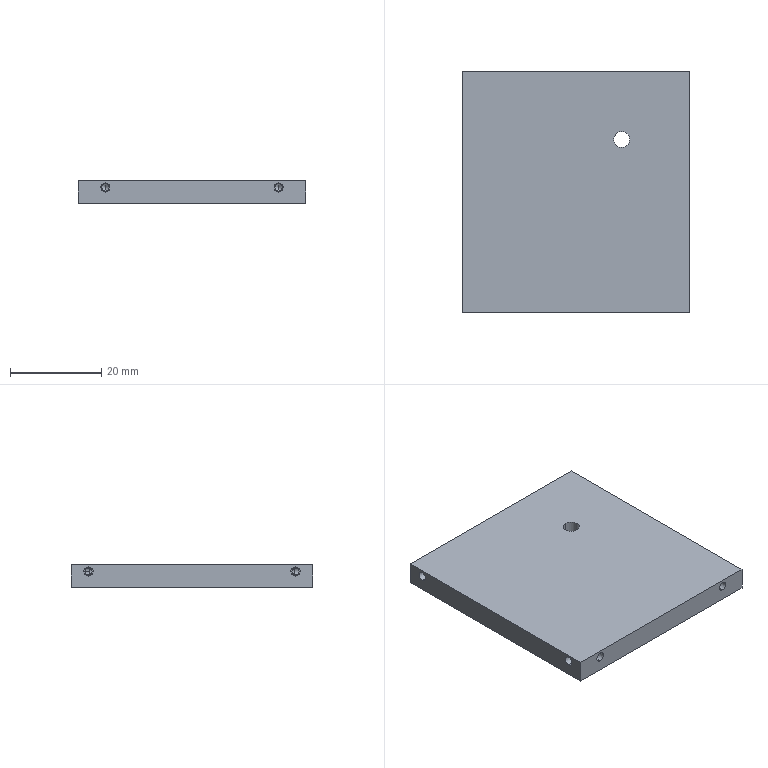Part | STEP file | ASND-0110-OPT-CO60-X-V1.0 rear cover plate | 1 solid | 68 faces | box 50 x 53 x 5 mm | volume 13081 mm3 | cylinder 34 | cone 20 | plane 14 | commonest cylinder face diameters 1.6 x16 2 x16 3.5 x2